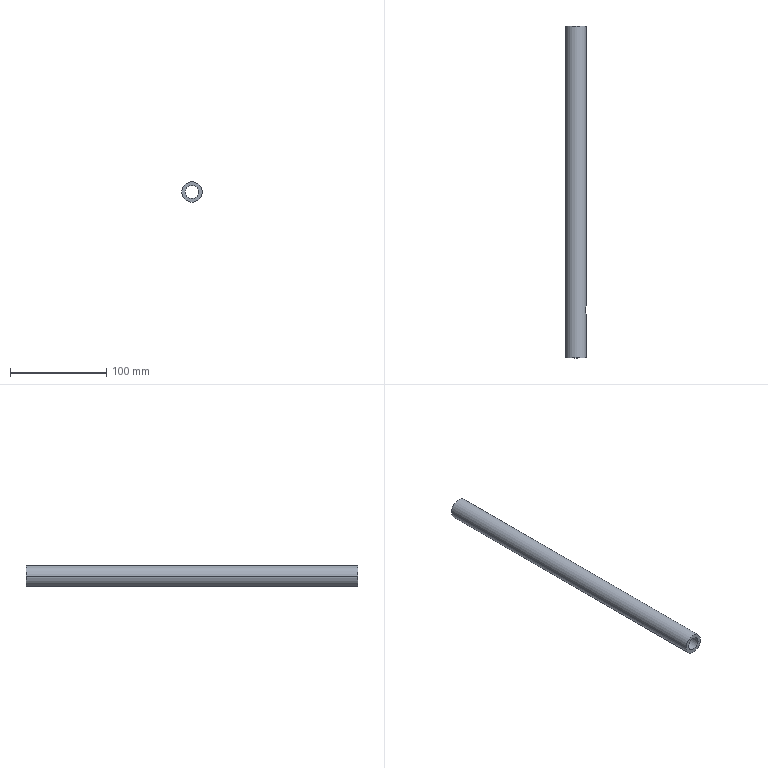Part | SolidWorks | features BaseBody 1 | 1 solid | 10 faces | box 21.234 x 344.346 x 21.234 mm | volume 69645 mm3 | cylinder 6 | plane 4 | commonest cylinder face diameters 10 x2 13.868 x2 21.234 x2
STEP:
#1=CARTESIAN_POINT('',(-28.118,-357.046,0.));
#2=VERTEX_POINT('',#1);
#3=CARTESIAN_POINT('',(-41.986,-357.046,0.));
#4=VERTEX_POINT('',#3);
#5=CARTESIAN_POINT('',(-35.052,-357.046,0.));
#6=DIRECTION('',(0.,-1.,0.));
#7=DIRECTION('',(1.,0.,0.));
#8=AXIS2_PLACEMENT_3D('',#5,#6,#7);
#9=CIRCLE('',#8,6.934);
#10=EDGE_CURVE('',#2,#4,#9,.T.);
#11=ORIENTED_EDGE('',*,*,#10,.F.);
#12=CARTESIAN_POINT('',(-35.052,-357.046,0.));
#13=DIRECTION('',(0.,-1.,0.));
#14=DIRECTION('',(-1.,0.,0.));
#15=AXIS2_PLACEMENT_3D('',#12,#13,#14);
#16=CIRCLE('',#15,6.934);
#17=EDGE_CURVE('',#4,#2,#16,.T.);
#18=ORIENTED_EDGE('',*,*,#17,.F.);
#19=EDGE_LOOP('',(#11,#18));
#20=FACE_BOUND('',#19,.T.);
#21=CARTESIAN_POINT('',(-24.435,-357.046,0.));
#22=VERTEX_POINT('',#21);
#23=CARTESIAN_POINT('',(-45.669,-357.046,0.));
#24=VERTEX_POINT('',#23);
#25=CARTESIAN_POINT('',(-35.052,-357.046,0.));
#26=DIRECTION('',(0.,1.,0.));
#27=DIRECTION('',(1.,0.,0.));
#28=AXIS2_PLACEMENT_3D('',#25,#26,#27);
#29=CIRCLE('',#28,10.617);
#30=EDGE_CURVE('',#22,#24,#29,.T.);
#31=ORIENTED_EDGE('',*,*,#30,.F.);
#32=CARTESIAN_POINT('',(-35.052,-357.046,0.));
#33=DIRECTION('',(0.,1.,0.));
#34=DIRECTION('',(-1.,0.,0.));
#35=AXIS2_PLACEMENT_3D('',#32,#33,#34);
#36=CIRCLE('',#35,10.617);
#37=EDGE_CURVE('',#24,#22,#36,.T.);
#38=ORIENTED_EDGE('',*,*,#37,.F.);
#39=EDGE_LOOP('',(#31,#38));
#40=FACE_OUTER_BOUND('',#39,.T.);
#41=CARTESIAN_POINT('',(-35.052,-357.046,0.));
#42=DIRECTION('',(0.,-1.,0.));
#43=DIRECTION('',(0.,0.,-1.));
#44=AXIS2_PLACEMENT_3D('',#41,#42,#43);
#45=PLANE('',#44);
#46=ADVANCED_FACE('',(#20,#40),#45,.T.);
#47=CARTESIAN_POINT('',(-28.118,-12.7,0.));
#48=VERTEX_POINT('',#47);
#49=CARTESIAN_POINT('',(-41.986,-12.7,0.));
#50=VERTEX_POINT('',#49);
#51=CARTESIAN_POINT('',(-35.052,-12.7,0.));
#52=DIRECTION('',(0.,1.,0.));
#53=DIRECTION('',(1.,0.,0.));
#54=AXIS2_PLACEMENT_3D('',#51,#52,#53);
#55=CIRCLE('',#54,6.934);
#56=EDGE_CURVE('',#48,#50,#55,.T.);
#57=ORIENTED_EDGE('',*,*,#56,.F.);
#58=CARTESIAN_POINT('',(-35.052,-12.7,0.));
#59=DIRECTION('',(0.,1.,0.));
#60=DIRECTION('',(-1.,0.,0.));
#61=AXIS2_PLACEMENT_3D('',#58,#59,#60);
#62=CIRCLE('',#61,6.934);
#63=EDGE_CURVE('',#50,#48,#62,.T.);
#64=ORIENTED_EDGE('',*,*,#63,.F.);
#65=EDGE_LOOP('',(#57,#64));
#66=FACE_BOUND('',#65,.T.);
#67=CARTESIAN_POINT('',(-24.435,-12.7,0.));
#68=VERTEX_POINT('',#67);
#69=CARTESIAN_POINT('',(-45.669,-12.7,0.));
#70=VERTEX_POINT('',#69);
#71=CARTESIAN_POINT('',(-35.052,-12.7,0.));
#72=DIRECTION('',(0.,-1.,0.));
#73=DIRECTION('',(1.,0.,0.));
#74=AXIS2_PLACEMENT_3D('',#71,#72,#73);
#75=CIRCLE('',#74,10.617);
#76=EDGE_CURVE('',#68,#70,#75,.T.);
#77=ORIENTED_EDGE('',*,*,#76,.F.);
#78=CARTESIAN_POINT('',(-35.052,-12.7,0.));
#79=DIRECTION('',(0.,-1.,0.));
#80=DIRECTION('',(-1.,0.,0.));
#81=AXIS2_PLACEMENT_3D('',#78,#79,#80);
#82=CIRCLE('',#81,10.617);
#83=EDGE_CURVE('',#70,#68,#82,.T.);
#84=ORIENTED_EDGE('',*,*,#83,.F.);
#85=EDGE_LOOP('',(#77,#84));
#86=FACE_OUTER_BOUND('',#85,.T.);
#87=CARTESIAN_POINT('',(-35.052,-12.7,0.));
#88=DIRECTION('',(0.,1.,0.));
#89=DIRECTION('',(1.,0.,0.));
#90=AXIS2_PLACEMENT_3D('',#87,#88,#89);
#91=PLANE('',#90);
#92=ADVANCED_FACE('',(#66,#86),#91,.T.);
#93=ORIENTED_EDGE('',*,*,#37,.T.);
#94=CARTESIAN_POINT('',(-24.435,-312.046,0.));
#95=VERTEX_POINT('',#94);
#96=CARTESIAN_POINT('',(-24.435,-312.046,0.));
#97=DIRECTION('',(0.,-1.,0.));
#98=VECTOR('',#97,1000.);
#99=LINE('',#96,#98);
#100=EDGE_CURVE('',#95,#22,#99,.T.);
#101=ORIENTED_EDGE('',*,*,#100,.F.);
#102=CARTESIAN_POINT('',(-25.686,-307.046,5.));
#103=VERTEX_POINT('',#102);
#104=CARTESIAN_POINT('',(-25.686,-307.046,5.));
#105=CARTESIAN_POINT('',(-25.686,-307.353,5.));
#106=CARTESIAN_POINT('',(-25.67,-307.672,4.972));
#107=CARTESIAN_POINT('',(-25.621,-308.157,4.878));
#108=CARTESIAN_POINT('',(-25.6,-308.32,4.838));
#109=CARTESIAN_POINT('',(-25.563,-308.565,4.765));
#110=CARTESIAN_POINT('',(-25.544,-308.687,4.724));
#111=CARTESIAN_POINT('',(-25.518,-308.829,4.671));
#112=CARTESIAN_POINT('',(-25.504,-308.9,4.643));
#113=CARTESIAN_POINT('',(-25.497,-308.936,4.629));
#114=CARTESIAN_POINT('',(-25.494,-308.954,4.622));
#115=CARTESIAN_POINT('',(-25.492,-308.961,4.619));
#116=CARTESIAN_POINT('',(-25.491,-308.966,4.617));
#117=CARTESIAN_POINT('',(-25.49,-308.97,4.615));
#118=CARTESIAN_POINT('',(-25.453,-309.154,4.538));
#119=CARTESIAN_POINT('',(-25.398,-309.391,4.428));
#120=CARTESIAN_POINT('',(-25.285,-309.806,4.173));
#121=CARTESIAN_POINT('',(-25.243,-309.953,4.072));
#122=CARTESIAN_POINT('',(-25.173,-310.183,3.894));
#123=CARTESIAN_POINT('',(-25.148,-310.261,3.83));
#124=CARTESIAN_POINT('',(-25.11,-310.38,3.727));
#125=CARTESIAN_POINT('',(-25.09,-310.439,3.673));
#126=CARTESIAN_POINT('',(-25.066,-310.509,3.607));
#127=CARTESIAN_POINT('',(-25.056,-310.539,3.578));
#128=CARTESIAN_POINT('',(-25.049,-310.559,3.558));
#129=CARTESIAN_POINT('',(-25.045,-310.57,3.547));
#130=CARTESIAN_POINT('',(-24.939,-310.869,3.248));
#131=CARTESIAN_POINT('',(-24.852,-311.094,2.953));
#132=CARTESIAN_POINT('',(-24.744,-311.355,2.542));
#133=CARTESIAN_POINT('',(-24.712,-311.43,2.409));
#134=CARTESIAN_POINT('',(-24.67,-311.526,2.221));
#135=CARTESIAN_POINT('',(-24.657,-311.556,2.16));
#136=CARTESIAN_POINT('',(-24.639,-311.597,2.071));
#137=CARTESIAN_POINT('',(-24.63,-311.617,2.028));
#138=CARTESIAN_POINT('',(-24.621,-311.638,1.978));
#139=CARTESIAN_POINT('',(-24.616,-311.649,1.953));
#140=CARTESIAN_POINT('',(-24.614,-311.653,1.943));
#141=CARTESIAN_POINT('',(-24.613,-311.656,1.936));
#142=CARTESIAN_POINT('',(-24.612,-311.657,1.934));
#143=CARTESIAN_POINT('',(-24.494,-311.925,1.292));
#144=CARTESIAN_POINT('',(-24.435,-312.046,0.6293));
#145=CARTESIAN_POINT('',(-24.435,-312.046,0.));
#146=B_SPLINE_CURVE_WITH_KNOTS('',3,(#104,#105,#106,#107,#108,#109,#110,#111,#112,#113,#114,#115,#116,#117,#118,#119,#120,#121,#122,#123,#124,#125,#126,#127,#128,#129,#130,#131,#132,#133,#134,#135,#136,#137,#138,#139,#140,#141,#142,#143,#144,#145),.UNSPECIFIED.,.F.,.F.,(4,2,2,1,1,1,1,1,2,2,2,2,2,1,1,2,2,2,2,2,1,1,1,2,2,4),(0.,0.125,0.1875,0.2187,0.2344,0.2422,0.2461,0.248,0.249,0.25,0.375,0.4375,0.4688,0.4844,0.4922,0.4961,0.5,0.625,0.6875,0.7188,0.7344,0.7422,0.7461,0.748,0.75,1.),.UNSPECIFIED.);
#147=EDGE_CURVE('',#103,#95,#146,.T.);
#148=ORIENTED_EDGE('',*,*,#147,.F.);
#149=CARTESIAN_POINT('',(-24.435,-302.046,0.));
#150=VERTEX_POINT('',#149);
#151=CARTESIAN_POINT('',(-24.435,-302.046,0.));
#152=CARTESIAN_POINT('',(-24.435,-302.046,0.3146));
#153=CARTESIAN_POINT('',(-24.45,-302.076,0.6371));
#154=CARTESIAN_POINT('',(-24.494,-302.171,1.123));
#155=CARTESIAN_POINT('',(-24.512,-302.211,1.285));
#156=CARTESIAN_POINT('',(-24.545,-302.284,1.528));
#157=CARTESIAN_POINT('',(-24.563,-302.324,1.649));
#158=CARTESIAN_POINT('',(-24.587,-302.377,1.789));
#159=CARTESIAN_POINT('',(-24.599,-302.404,1.859));
#160=CARTESIAN_POINT('',(-24.605,-302.419,1.894));
#161=CARTESIAN_POINT('',(-24.608,-302.425,1.909));
#162=CARTESIAN_POINT('',(-24.61,-302.429,1.919));
#163=CARTESIAN_POINT('',(-24.611,-302.432,1.926));
#164=CARTESIAN_POINT('',(-24.652,-302.525,2.15));
#165=CARTESIAN_POINT('',(-24.709,-302.65,2.404));
#166=CARTESIAN_POINT('',(-24.816,-302.911,2.816));
#167=CARTESIAN_POINT('',(-24.856,-303.011,2.958));
#168=CARTESIAN_POINT('',(-24.921,-303.182,3.175));
#169=CARTESIAN_POINT('',(-24.944,-303.243,3.247));
#170=CARTESIAN_POINT('',(-24.98,-303.34,3.356));
#171=CARTESIAN_POINT('',(-24.998,-303.39,3.411));
#172=CARTESIAN_POINT('',(-25.019,-303.45,3.475));
#173=CARTESIAN_POINT('',(-25.029,-303.477,3.502));
#174=CARTESIAN_POINT('',(-25.035,-303.495,3.52));
#175=CARTESIAN_POINT('',(-25.038,-303.503,3.528));
#176=CARTESIAN_POINT('',(-25.154,-303.832,3.857));
#177=CARTESIAN_POINT('',(-25.248,-304.148,4.087));
#178=CARTESIAN_POINT('',(-25.36,-304.562,4.343));
#179=CARTESIAN_POINT('',(-25.393,-304.691,4.413));
#180=CARTESIAN_POINT('',(-25.435,-304.866,4.5));
#181=CARTESIAN_POINT('',(-25.447,-304.922,4.527));
#182=CARTESIAN_POINT('',(-25.465,-305.,4.562));
#183=CARTESIAN_POINT('',(-25.473,-305.038,4.579));
#184=CARTESIAN_POINT('',(-25.482,-305.08,4.597));
#185=CARTESIAN_POINT('',(-25.486,-305.1,4.606));
#186=CARTESIAN_POINT('',(-25.488,-305.111,4.61));
#187=CARTESIAN_POINT('',(-25.489,-305.115,4.612));
#188=CARTESIAN_POINT('',(-25.489,-305.118,4.613));
#189=CARTESIAN_POINT('',(-25.489,-305.118,4.613));
#190=CARTESIAN_POINT('',(-25.621,-305.769,4.885));
#191=CARTESIAN_POINT('',(-25.686,-306.431,5.));
#192=CARTESIAN_POINT('',(-25.686,-307.046,5.));
#193=B_SPLINE_CURVE_WITH_KNOTS('',3,(#151,#152,#153,#154,#155,#156,#157,#158,#159,#160,#161,#162,#163,#164,#165,#166,#167,#168,#169,#170,#171,#172,#173,#174,#175,#176,#177,#178,#179,#180,#181,#182,#183,#184,#185,#186,#187,#188,#189,#190,#191,#192),.UNSPECIFIED.,.F.,.F.,(4,2,2,1,1,1,1,2,2,2,2,2,1,1,2,2,2,2,2,1,1,1,1,2,2,4),(0.,0.125,0.1875,0.2188,0.2344,0.2422,0.2461,0.248,0.25,0.375,0.4375,0.4688,0.4844,0.4922,0.4961,0.5,0.625,0.6875,0.7188,0.7344,0.7422,0.7461,0.748,0.749,0.75,1.),.UNSPECIFIED.);
#194=EDGE_CURVE('',#150,#103,#193,.T.);
#195=ORIENTED_EDGE('',*,*,#194,.F.);
#196=CARTESIAN_POINT('',(-24.435,-12.7,0.));
#197=DIRECTION('',(0.,-1.,0.));
#198=VECTOR('',#197,1000.);
#199=LINE('',#196,#198);
#200=EDGE_CURVE('',#68,#150,#199,.T.);
#201=ORIENTED_EDGE('',*,*,#200,.F.);
#202=ORIENTED_EDGE('',*,*,#76,.T.);
#203=CARTESIAN_POINT('',(-45.669,-357.046,0.));
#204=DIRECTION('',(0.,1.,0.));
#205=VECTOR('',#204,1000.);
#206=LINE('',#203,#205);
#207=EDGE_CURVE('',#24,#70,#206,.T.);
#208=ORIENTED_EDGE('',*,*,#207,.F.);
#209=EDGE_LOOP('',(#93,#101,#148,#195,#201,#202,#208));
#210=FACE_OUTER_BOUND('',#209,.T.);
#211=CARTESIAN_POINT('',(-35.052,-12.7,0.));
#212=DIRECTION('',(0.,-1.,0.));
#213=DIRECTION('',(1.,0.,0.));
#214=AXIS2_PLACEMENT_3D('',#211,#212,#213);
#215=CYLINDRICAL_SURFACE('',#214,10.617);
#216=ADVANCED_FACE('',(#210),#215,.T.);
#217=ORIENTED_EDGE('',*,*,#207,.T.);
#218=ORIENTED_EDGE('',*,*,#83,.T.);
#219=ORIENTED_EDGE('',*,*,#200,.T.);
#220=CARTESIAN_POINT('',(-25.686,-307.046,-5.));
#221=VERTEX_POINT('',#220);
#222=CARTESIAN_POINT('',(-25.686,-307.046,-5.));
#223=CARTESIAN_POINT('',(-25.686,-306.739,-5.));
#224=CARTESIAN_POINT('',(-25.67,-306.42,-4.972));
#225=CARTESIAN_POINT('',(-25.621,-305.935,-4.878));
#226=CARTESIAN_POINT('',(-25.6,-305.772,-4.838));
#227=CARTESIAN_POINT('',(-25.563,-305.527,-4.765));
#228=CARTESIAN_POINT('',(-25.544,-305.405,-4.724));
#229=CARTESIAN_POINT('',(-25.518,-305.263,-4.671));
#230=CARTESIAN_POINT('',(-25.504,-305.192,-4.643));
#231=CARTESIAN_POINT('',(-25.497,-305.156,-4.629));
#232=CARTESIAN_POINT('',(-25.494,-305.138,-4.622));
#233=CARTESIAN_POINT('',(-25.492,-305.131,-4.619));
#234=CARTESIAN_POINT('',(-25.491,-305.126,-4.617));
#235=CARTESIAN_POINT('',(-25.49,-305.122,-4.615));
#236=CARTESIAN_POINT('',(-25.453,-304.938,-4.538));
#237=CARTESIAN_POINT('',(-25.398,-304.701,-4.428));
#238=CARTESIAN_POINT('',(-25.285,-304.286,-4.173));
#239=CARTESIAN_POINT('',(-25.243,-304.139,-4.072));
#240=CARTESIAN_POINT('',(-25.173,-303.909,-3.894));
#241=CARTESIAN_POINT('',(-25.148,-303.831,-3.83));
#242=CARTESIAN_POINT('',(-25.11,-303.712,-3.727));
#243=CARTESIAN_POINT('',(-25.09,-303.653,-3.673));
#244=CARTESIAN_POINT('',(-25.066,-303.583,-3.607));
#245=CARTESIAN_POINT('',(-25.056,-303.553,-3.578));
#246=CARTESIAN_POINT('',(-25.049,-303.533,-3.558));
#247=CARTESIAN_POINT('',(-25.045,-303.522,-3.547));
#248=CARTESIAN_POINT('',(-24.939,-303.223,-3.248));
#249=CARTESIAN_POINT('',(-24.852,-302.998,-2.953));
#250=CARTESIAN_POINT('',(-24.744,-302.737,-2.542));
#251=CARTESIAN_POINT('',(-24.712,-302.662,-2.409));
#252=CARTESIAN_POINT('',(-24.67,-302.566,-2.221));
#253=CARTESIAN_POINT('',(-24.657,-302.536,-2.16));
#254=CARTESIAN_POINT('',(-24.639,-302.495,-2.071));
#255=CARTESIAN_POINT('',(-24.63,-302.475,-2.028));
#256=CARTESIAN_POINT('',(-24.621,-302.454,-1.978));
#257=CARTESIAN_POINT('',(-24.616,-302.443,-1.953));
#258=CARTESIAN_POINT('',(-24.614,-302.439,-1.943));
#259=CARTESIAN_POINT('',(-24.613,-302.436,-1.936));
#260=CARTESIAN_POINT('',(-24.612,-302.435,-1.934));
#261=CARTESIAN_POINT('',(-24.494,-302.167,-1.292));
#262=CARTESIAN_POINT('',(-24.435,-302.046,-0.6293));
#263=CARTESIAN_POINT('',(-24.435,-302.046,0.));
#264=B_SPLINE_CURVE_WITH_KNOTS('',3,(#222,#223,#224,#225,#226,#227,#228,#229,#230,#231,#232,#233,#234,#235,#236,#237,#238,#239,#240,#241,#242,#243,#244,#245,#246,#247,#248,#249,#250,#251,#252,#253,#254,#255,#256,#257,#258,#259,#260,#261,#262,#263),.UNSPECIFIED.,.F.,.F.,(4,2,2,1,1,1,1,1,2,2,2,2,2,1,1,2,2,2,2,2,1,1,1,2,2,4),(0.,0.125,0.1875,0.2188,0.2344,0.2422,0.2461,0.248,0.249,0.25,0.375,0.4375,0.4688,0.4844,0.4922,0.4961,0.5,0.625,0.6875,0.7188,0.7344,0.7422,0.7461,0.748,0.75,1.),.UNSPECIFIED.);
#265=EDGE_CURVE('',#221,#150,#264,.T.);
#266=ORIENTED_EDGE('',*,*,#265,.F.);
#267=CARTESIAN_POINT('',(-24.435,-312.046,0.));
#268=CARTESIAN_POINT('',(-24.435,-312.046,-0.3146));
#269=CARTESIAN_POINT('',(-24.45,-312.016,-0.6371));
#270=CARTESIAN_POINT('',(-24.494,-311.921,-1.123));
#271=CARTESIAN_POINT('',(-24.512,-311.881,-1.285));
#272=CARTESIAN_POINT('',(-24.545,-311.808,-1.528));
#273=CARTESIAN_POINT('',(-24.563,-311.768,-1.649));
#274=CARTESIAN_POINT('',(-24.587,-311.715,-1.789));
#275=CARTESIAN_POINT('',(-24.599,-311.688,-1.859));
#276=CARTESIAN_POINT('',(-24.605,-311.673,-1.894));
#277=CARTESIAN_POINT('',(-24.608,-311.667,-1.909));
#278=CARTESIAN_POINT('',(-24.61,-311.663,-1.919));
#279=CARTESIAN_POINT('',(-24.611,-311.66,-1.926));
#280=CARTESIAN_POINT('',(-24.652,-311.567,-2.15));
#281=CARTESIAN_POINT('',(-24.709,-311.442,-2.404));
#282=CARTESIAN_POINT('',(-24.816,-311.181,-2.816));
#283=CARTESIAN_POINT('',(-24.856,-311.081,-2.958));
#284=CARTESIAN_POINT('',(-24.921,-310.91,-3.175));
#285=CARTESIAN_POINT('',(-24.944,-310.849,-3.247));
#286=CARTESIAN_POINT('',(-24.98,-310.752,-3.356));
#287=CARTESIAN_POINT('',(-24.998,-310.702,-3.411));
#288=CARTESIAN_POINT('',(-25.019,-310.642,-3.475));
#289=CARTESIAN_POINT('',(-25.029,-310.615,-3.502));
#290=CARTESIAN_POINT('',(-25.035,-310.597,-3.52));
#291=CARTESIAN_POINT('',(-25.038,-310.589,-3.528));
#292=CARTESIAN_POINT('',(-25.154,-310.26,-3.857));
#293=CARTESIAN_POINT('',(-25.248,-309.944,-4.087));
#294=CARTESIAN_POINT('',(-25.36,-309.53,-4.343));
#295=CARTESIAN_POINT('',(-25.393,-309.401,-4.413));
#296=CARTESIAN_POINT('',(-25.435,-309.226,-4.5));
#297=CARTESIAN_POINT('',(-25.447,-309.17,-4.527));
#298=CARTESIAN_POINT('',(-25.465,-309.092,-4.562));
#299=CARTESIAN_POINT('',(-25.473,-309.054,-4.579));
#300=CARTESIAN_POINT('',(-25.482,-309.012,-4.597));
#301=CARTESIAN_POINT('',(-25.486,-308.992,-4.606));
#302=CARTESIAN_POINT('',(-25.488,-308.981,-4.61));
#303=CARTESIAN_POINT('',(-25.489,-308.977,-4.612));
#304=CARTESIAN_POINT('',(-25.489,-308.974,-4.613));
#305=CARTESIAN_POINT('',(-25.489,-308.974,-4.613));
#306=CARTESIAN_POINT('',(-25.621,-308.323,-4.885));
#307=CARTESIAN_POINT('',(-25.686,-307.661,-5.));
#308=CARTESIAN_POINT('',(-25.686,-307.046,-5.));
#309=B_SPLINE_CURVE_WITH_KNOTS('',3,(#267,#268,#269,#270,#271,#272,#273,#274,#275,#276,#277,#278,#279,#280,#281,#282,#283,#284,#285,#286,#287,#288,#289,#290,#291,#292,#293,#294,#295,#296,#297,#298,#299,#300,#301,#302,#303,#304,#305,#306,#307,#308),.UNSPECIFIED.,.F.,.F.,(4,2,2,1,1,1,1,2,2,2,2,2,1,1,2,2,2,2,2,1,1,1,1,2,2,4),(0.,0.125,0.1875,0.2187,0.2344,0.2422,0.2461,0.248,0.25,0.375,0.4375,0.4687,0.4844,0.4922,0.4961,0.5,0.625,0.6875,0.7187,0.7344,0.7422,0.7461,0.748,0.749,0.75,1.),.UNSPECIFIED.);
#310=EDGE_CURVE('',#95,#221,#309,.T.);
#311=ORIENTED_EDGE('',*,*,#310,.F.);
#312=ORIENTED_EDGE('',*,*,#100,.T.);
#313=ORIENTED_EDGE('',*,*,#30,.T.);
#314=EDGE_LOOP('',(#217,#218,#219,#266,#311,#312,#313));
#315=FACE_OUTER_BOUND('',#314,.T.);
#316=CARTESIAN_POINT('',(-35.052,-12.7,0.));
#317=DIRECTION('',(0.,-1.,0.));
#318=DIRECTION('',(1.,0.,0.));
#319=AXIS2_PLACEMENT_3D('',#316,#317,#318);
#320=CYLINDRICAL_SURFACE('',#319,10.617);
#321=ADVANCED_FACE('',(#315),#320,.T.);
#322=ORIENTED_EDGE('',*,*,#17,.T.);
#323=CARTESIAN_POINT('',(-28.118,-312.046,-0.000000001));
#324=VERTEX_POINT('',#323);
#325=CARTESIAN_POINT('',(-28.118,-312.046,0.));
#326=DIRECTION('',(0.,-1.,0.));
#327=VECTOR('',#326,1000.);
#328=LINE('',#325,#327);
#329=EDGE_CURVE('',#324,#2,#328,.T.);
#330=ORIENTED_EDGE('',*,*,#329,.F.);
#331=CARTESIAN_POINT('',(-28.435,-311.596,-2.073));
#332=VERTEX_POINT('',#331);
#333=CARTESIAN_POINT('',(-28.435,-311.596,-2.073));
#334=CARTESIAN_POINT('',(-28.223,-311.904,-1.398));
#335=CARTESIAN_POINT('',(-28.118,-312.046,-0.6833));
#336=CARTESIAN_POINT('',(-28.118,-312.046,-0.000000001));
#337=B_SPLINE_CURVE_WITH_KNOTS('',3,(#333,#334,#335,#336),.UNSPECIFIED.,.F.,.F.,(4,4),(0.,1.),.UNSPECIFIED.);
#338=EDGE_CURVE('',#332,#324,#337,.T.);
#339=ORIENTED_EDGE('',*,*,#338,.F.);
#340=CARTESIAN_POINT('',(-28.435,-302.496,-2.073));
#341=VERTEX_POINT('',#340);
#342=CARTESIAN_POINT('',(-28.435,-302.496,-2.073));
#343=DIRECTION('',(0.,-1.,0.));
#344=VECTOR('',#343,1000.);
#345=LINE('',#342,#344);
#346=EDGE_CURVE('',#341,#332,#345,.T.);
#347=ORIENTED_EDGE('',*,*,#346,.F.);
#348=CARTESIAN_POINT('',(-28.118,-302.046,0.000000001));
#349=VERTEX_POINT('',#348);
#350=CARTESIAN_POINT('',(-28.118,-302.046,0.000000001));
#351=CARTESIAN_POINT('',(-28.118,-302.046,-0.6833));
#352=CARTESIAN_POINT('',(-28.223,-302.188,-1.398));
#353=CARTESIAN_POINT('',(-28.435,-302.496,-2.073));
#354=B_SPLINE_CURVE_WITH_KNOTS('',3,(#350,#351,#352,#353),.UNSPECIFIED.,.F.,.F.,(4,4),(0.,1.),.UNSPECIFIED.);
#355=EDGE_CURVE('',#349,#341,#354,.T.);
#356=ORIENTED_EDGE('',*,*,#355,.F.);
#357=CARTESIAN_POINT('',(-28.118,-12.7,0.));
#358=DIRECTION('',(0.,-1.,0.));
#359=VECTOR('',#358,1000.);
#360=LINE('',#357,#359);
#361=EDGE_CURVE('',#48,#349,#360,.T.);
#362=ORIENTED_EDGE('',*,*,#361,.F.);
#363=ORIENTED_EDGE('',*,*,#56,.T.);
#364=CARTESIAN_POINT('',(-41.986,-357.046,0.));
#365=DIRECTION('',(0.,1.,0.));
#366=VECTOR('',#365,1000.);
#367=LINE('',#364,#366);
#368=EDGE_CURVE('',#4,#50,#367,.T.);
#369=ORIENTED_EDGE('',*,*,#368,.F.);
#370=EDGE_LOOP('',(#322,#330,#339,#347,#356,#362,#363,#369));
#371=FACE_OUTER_BOUND('',#370,.T.);
#372=CARTESIAN_POINT('',(-35.052,-12.7,0.));
#373=DIRECTION('',(0.,-1.,0.));
#374=DIRECTION('',(1.,0.,0.));
#375=AXIS2_PLACEMENT_3D('',#372,#373,#374);
#376=CYLINDRICAL_SURFACE('',#375,6.934);
#377=ADVANCED_FACE('',(#371),#376,.F.);
#378=ORIENTED_EDGE('',*,*,#368,.T.);
#379=ORIENTED_EDGE('',*,*,#63,.T.);
#380=ORIENTED_EDGE('',*,*,#361,.T.);
#381=CARTESIAN_POINT('',(-28.435,-302.496,2.073));
#382=VERTEX_POINT('',#381);
#383=CARTESIAN_POINT('',(-28.435,-302.496,2.073));
#384=CARTESIAN_POINT('',(-28.223,-302.188,1.398));
#385=CARTESIAN_POINT('',(-28.118,-302.046,0.6833));
#386=CARTESIAN_POINT('',(-28.118,-302.046,0.000000001));
#387=B_SPLINE_CURVE_WITH_KNOTS('',3,(#383,#384,#385,#386),.UNSPECIFIED.,.F.,.F.,(4,4),(0.,1.),.UNSPECIFIED.);
#388=EDGE_CURVE('',#382,#349,#387,.T.);
#389=ORIENTED_EDGE('',*,*,#388,.F.);
#390=CARTESIAN_POINT('',(-28.435,-311.596,2.073));
#391=VERTEX_POINT('',#390);
#392=CARTESIAN_POINT('',(-28.435,-311.596,2.073));
#393=DIRECTION('',(0.,1.,0.));
#394=VECTOR('',#393,1000.);
#395=LINE('',#392,#394);
#396=EDGE_CURVE('',#391,#382,#395,.T.);
#397=ORIENTED_EDGE('',*,*,#396,.F.);
#398=CARTESIAN_POINT('',(-28.118,-312.046,-0.000000001));
#399=CARTESIAN_POINT('',(-28.118,-312.046,0.6833));
#400=CARTESIAN_POINT('',(-28.223,-311.904,1.398));
#401=CARTESIAN_POINT('',(-28.435,-311.596,2.073));
#402=B_SPLINE_CURVE_WITH_KNOTS('',3,(#398,#399,#400,#401),.UNSPECIFIED.,.F.,.F.,(4,4),(0.,1.),.UNSPECIFIED.);
#403=EDGE_CURVE('',#324,#391,#402,.T.);
#404=ORIENTED_EDGE('',*,*,#403,.F.);
#405=ORIENTED_EDGE('',*,*,#329,.T.);
#406=ORIENTED_EDGE('',*,*,#10,.T.);
#407=EDGE_LOOP('',(#378,#379,#380,#389,#397,#404,#405,#406));
#408=FACE_OUTER_BOUND('',#407,.T.);
#409=CARTESIAN_POINT('',(-35.052,-12.7,0.));
#410=DIRECTION('',(0.,-1.,0.));
#411=DIRECTION('',(1.,0.,0.));
#412=AXIS2_PLACEMENT_3D('',#409,#410,#411);
#413=CYLINDRICAL_SURFACE('',#412,6.934);
#414=ADVANCED_FACE('',(#408),#413,.F.);
#415=ORIENTED_EDGE('',*,*,#396,.T.);
#416=CARTESIAN_POINT('',(-28.435,-307.046,5.));
#417=VERTEX_POINT('',#416);
#418=CARTESIAN_POINT('',(-28.435,-307.046,0.));
#419=DIRECTION('',(-1.,0.,0.));
#420=DIRECTION('',(0.,0.,1.));
#421=AXIS2_PLACEMENT_3D('',#418,#419,#420);
#422=CIRCLE('',#421,5.);
#423=EDGE_CURVE('',#417,#382,#422,.T.);
#424=ORIENTED_EDGE('',*,*,#423,.F.);
#425=CARTESIAN_POINT('',(-28.435,-307.046,0.));
#426=DIRECTION('',(-1.,0.,0.));
#427=DIRECTION('',(0.,-0.91,0.4145));
#428=AXIS2_PLACEMENT_3D('',#425,#426,#427);
#429=CIRCLE('',#428,5.);
#430=EDGE_CURVE('',#391,#417,#429,.T.);
#431=ORIENTED_EDGE('',*,*,#430,.F.);
#432=EDGE_LOOP('',(#415,#424,#431));
#433=FACE_OUTER_BOUND('',#432,.T.);
#434=CARTESIAN_POINT('',(-28.435,-307.046,0.));
#435=DIRECTION('',(1.,0.,0.));
#436=DIRECTION('',(0.,1.,0.));
#437=AXIS2_PLACEMENT_3D('',#434,#435,#436);
#438=PLANE('',#437);
#439=ADVANCED_FACE('',(#433),#438,.T.);
#440=ORIENTED_EDGE('',*,*,#147,.T.);
#441=ORIENTED_EDGE('',*,*,#310,.T.);
#442=CARTESIAN_POINT('',(-28.435,-307.046,-5.));
#443=VERTEX_POINT('',#442);
#444=CARTESIAN_POINT('',(-28.435,-307.046,-5.));
#445=DIRECTION('',(1.,0.,0.));
#446=VECTOR('',#445,1000.);
#447=LINE('',#444,#446);
#448=EDGE_CURVE('',#443,#221,#447,.T.);
#449=ORIENTED_EDGE('',*,*,#448,.F.);
#450=CARTESIAN_POINT('',(-28.435,-307.046,0.));
#451=DIRECTION('',(1.,0.,0.));
#452=DIRECTION('',(0.,-0.91,-0.4145));
#453=AXIS2_PLACEMENT_3D('',#450,#451,#452);
#454=CIRCLE('',#453,5.);
#455=EDGE_CURVE('',#332,#443,#454,.T.);
#456=ORIENTED_EDGE('',*,*,#455,.F.);
#457=ORIENTED_EDGE('',*,*,#338,.T.);
#458=ORIENTED_EDGE('',*,*,#403,.T.);
#459=ORIENTED_EDGE('',*,*,#430,.T.);
#460=CARTESIAN_POINT('',(-25.686,-307.046,5.));
#461=DIRECTION('',(-1.,0.,0.));
#462=VECTOR('',#461,1000.);
#463=LINE('',#460,#462);
#464=EDGE_CURVE('',#103,#417,#463,.T.);
#465=ORIENTED_EDGE('',*,*,#464,.F.);
#466=EDGE_LOOP('',(#440,#441,#449,#456,#457,#458,#459,#465));
#467=FACE_OUTER_BOUND('',#466,.T.);
#468=CARTESIAN_POINT('',(-24.435,-307.046,0.));
#469=DIRECTION('',(-1.,0.,0.));
#470=DIRECTION('',(0.,0.,-1.));
#471=AXIS2_PLACEMENT_3D('',#468,#469,#470);
#472=CYLINDRICAL_SURFACE('',#471,5.);
#473=ADVANCED_FACE('',(#467),#472,.F.);
#474=ORIENTED_EDGE('',*,*,#194,.T.);
#475=ORIENTED_EDGE('',*,*,#464,.T.);
#476=ORIENTED_EDGE('',*,*,#423,.T.);
#477=ORIENTED_EDGE('',*,*,#388,.T.);
#478=ORIENTED_EDGE('',*,*,#355,.T.);
#479=CARTESIAN_POINT('',(-28.435,-307.046,0.));
#480=DIRECTION('',(1.,0.,0.));
#481=DIRECTION('',(0.,0.,-1.));
#482=AXIS2_PLACEMENT_3D('',#479,#480,#481);
#483=CIRCLE('',#482,5.);
#484=EDGE_CURVE('',#443,#341,#483,.T.);
#485=ORIENTED_EDGE('',*,*,#484,.F.);
#486=ORIENTED_EDGE('',*,*,#448,.T.);
#487=ORIENTED_EDGE('',*,*,#265,.T.);
#488=EDGE_LOOP('',(#474,#475,#476,#477,#478,#485,#486,#487));
#489=FACE_OUTER_BOUND('',#488,.T.);
#490=CARTESIAN_POINT('',(-24.435,-307.046,0.));
#491=DIRECTION('',(-1.,0.,0.));
#492=DIRECTION('',(0.,0.,-1.));
#493=AXIS2_PLACEMENT_3D('',#490,#491,#492);
#494=CYLINDRICAL_SURFACE('',#493,5.);
#495=ADVANCED_FACE('',(#489),#494,.F.);
#496=ORIENTED_EDGE('',*,*,#346,.T.);
#497=ORIENTED_EDGE('',*,*,#455,.T.);
#498=ORIENTED_EDGE('',*,*,#484,.T.);
#499=EDGE_LOOP('',(#496,#497,#498));
#500=FACE_OUTER_BOUND('',#499,.T.);
#501=CARTESIAN_POINT('',(-28.435,-307.046,0.));
#502=DIRECTION('',(1.,0.,0.));
#503=DIRECTION('',(0.,1.,0.));
#504=AXIS2_PLACEMENT_3D('',#501,#502,#503);
#505=PLANE('',#504);
#506=ADVANCED_FACE('',(#500),#505,.T.);
#507=CLOSED_SHELL('',(#46,#92,#216,#321,#377,#414,#439,#473,#495,#506));
#508=MANIFOLD_SOLID_BREP('',#507);
#509=CARTESIAN_POINT('',(0.,0.,0.));
#510=DIRECTION('',(0.,0.,1.));
#511=DIRECTION('',(1.,0.,0.));
#512=AXIS2_PLACEMENT_3D('',#509,#510,#511);
#513=(LENGTH_UNIT()NAMED_UNIT(*)SI_UNIT(.MILLI.,.METRE.));
#514=UNCERTAINTY_MEASURE_WITH_UNIT(LENGTH_MEASURE(0.00001),#513,'','');
#515=(NAMED_UNIT(*)PLANE_ANGLE_UNIT()SI_UNIT($,.RADIAN.));
#516=(NAMED_UNIT(*)SI_UNIT($,.STERADIAN.)SOLID_ANGLE_UNIT());
#517=(GEOMETRIC_REPRESENTATION_CONTEXT(3)GLOBAL_UNCERTAINTY_ASSIGNED_CONTEXT((#514))GLOBAL_UNIT_ASSIGNED_CONTEXT((#513,#515,#516))REPRESENTATION_CONTEXT('',''));
#518=ADVANCED_BREP_SHAPE_REPRESENTATION('',(#508,#512),#517);